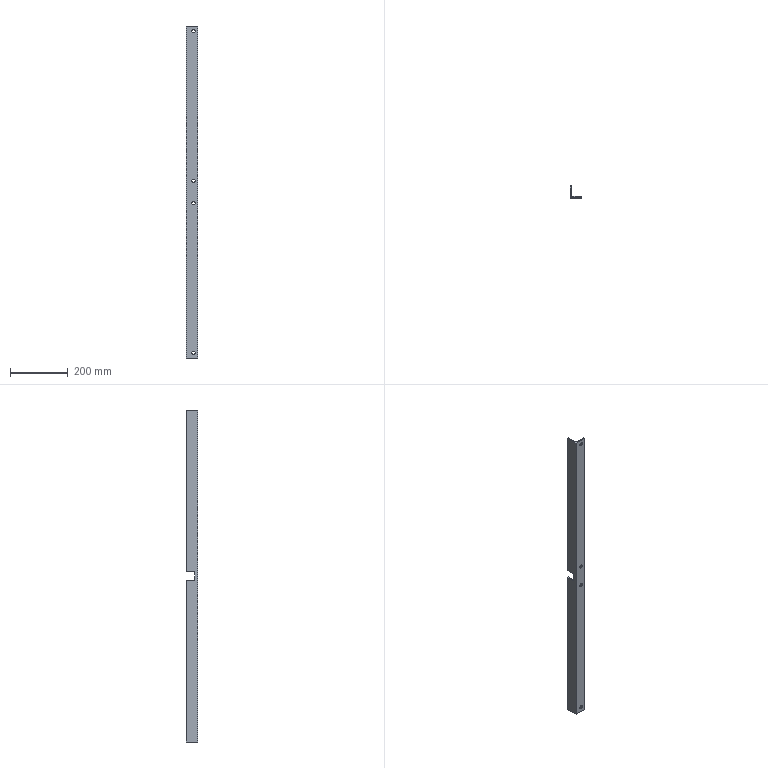Part | SolidWorks | features Extrusion 1, HoleWzd 1, ICE 1 | 1 solid | 24 faces | box 40 x 40 x 1150 mm | volume 350360 mm3 | cylinder 12 | plane 12 | commonest cylinder face diameters 12 x8 0.02 x3 10 x1
STEP:
#1=CARTESIAN_POINT('',(24.99,0.,1126.));
#2=VERTEX_POINT('',#1);
#3=CARTESIAN_POINT('',(24.99,0.,1138.));
#4=VERTEX_POINT('',#3);
#5=CARTESIAN_POINT('',(24.99,0.,1132.));
#6=DIRECTION('',(0.,1.,0.));
#7=DIRECTION('',(0.,0.,1.));
#8=AXIS2_PLACEMENT_3D('',#5,#6,#7);
#9=CIRCLE('',#8,6.);
#10=EDGE_CURVE('',#2,#4,#9,.T.);
#11=ORIENTED_EDGE('',*,*,#10,.F.);
#12=CARTESIAN_POINT('',(24.99,4.,1126.));
#13=VERTEX_POINT('',#12);
#14=CARTESIAN_POINT('',(24.99,4.,1126.));
#15=DIRECTION('',(0.,1.,0.));
#16=VECTOR('',#15,1000.);
#17=LINE('',#14,#16);
#18=EDGE_CURVE('',#2,#13,#17,.T.);
#19=ORIENTED_EDGE('',*,*,#18,.T.);
#20=CARTESIAN_POINT('',(24.99,4.,1138.));
#21=VERTEX_POINT('',#20);
#22=CARTESIAN_POINT('',(24.99,4.,1132.));
#23=DIRECTION('',(0.,1.,0.));
#24=DIRECTION('',(0.,0.,1.));
#25=AXIS2_PLACEMENT_3D('',#22,#23,#24);
#26=CIRCLE('',#25,6.);
#27=EDGE_CURVE('',#13,#21,#26,.T.);
#28=ORIENTED_EDGE('',*,*,#27,.T.);
#29=CARTESIAN_POINT('',(24.99,4.,1138.));
#30=DIRECTION('',(0.,1.,0.));
#31=VECTOR('',#30,1000.);
#32=LINE('',#29,#31);
#33=EDGE_CURVE('',#4,#21,#32,.T.);
#34=ORIENTED_EDGE('',*,*,#33,.F.);
#35=EDGE_LOOP('',(#11,#19,#28,#34));
#36=FACE_OUTER_BOUND('',#35,.T.);
#37=CARTESIAN_POINT('',(24.99,4.,1132.));
#38=DIRECTION('',(0.,1.,0.));
#39=DIRECTION('',(0.,0.,1.));
#40=AXIS2_PLACEMENT_3D('',#37,#38,#39);
#41=CYLINDRICAL_SURFACE('',#40,6.);
#42=ADVANCED_FACE('',(#36),#41,.F.);
#43=CARTESIAN_POINT('',(24.99,0.,608.));
#44=VERTEX_POINT('',#43);
#45=CARTESIAN_POINT('',(24.99,0.,620.));
#46=VERTEX_POINT('',#45);
#47=CARTESIAN_POINT('',(24.99,0.,614.));
#48=DIRECTION('',(0.,1.,0.));
#49=DIRECTION('',(0.,0.,1.));
#50=AXIS2_PLACEMENT_3D('',#47,#48,#49);
#51=CIRCLE('',#50,6.);
#52=EDGE_CURVE('',#44,#46,#51,.T.);
#53=ORIENTED_EDGE('',*,*,#52,.F.);
#54=CARTESIAN_POINT('',(24.99,4.,608.));
#55=VERTEX_POINT('',#54);
#56=CARTESIAN_POINT('',(24.99,4.,608.));
#57=DIRECTION('',(0.,1.,0.));
#58=VECTOR('',#57,1000.);
#59=LINE('',#56,#58);
#60=EDGE_CURVE('',#44,#55,#59,.T.);
#61=ORIENTED_EDGE('',*,*,#60,.T.);
#62=CARTESIAN_POINT('',(24.99,4.,620.));
#63=VERTEX_POINT('',#62);
#64=CARTESIAN_POINT('',(24.99,4.,614.));
#65=DIRECTION('',(0.,1.,0.));
#66=DIRECTION('',(0.,0.,1.));
#67=AXIS2_PLACEMENT_3D('',#64,#65,#66);
#68=CIRCLE('',#67,6.);
#69=EDGE_CURVE('',#55,#63,#68,.T.);
#70=ORIENTED_EDGE('',*,*,#69,.T.);
#71=CARTESIAN_POINT('',(24.99,4.,620.));
#72=DIRECTION('',(0.,1.,0.));
#73=VECTOR('',#72,1000.);
#74=LINE('',#71,#73);
#75=EDGE_CURVE('',#46,#63,#74,.T.);
#76=ORIENTED_EDGE('',*,*,#75,.F.);
#77=EDGE_LOOP('',(#53,#61,#70,#76));
#78=FACE_OUTER_BOUND('',#77,.T.);
#79=CARTESIAN_POINT('',(24.99,4.,614.));
#80=DIRECTION('',(0.,1.,0.));
#81=DIRECTION('',(0.,0.,1.));
#82=AXIS2_PLACEMENT_3D('',#79,#80,#81);
#83=CYLINDRICAL_SURFACE('',#82,6.);
#84=ADVANCED_FACE('',(#78),#83,.F.);
#85=CARTESIAN_POINT('',(24.99,0.,530.));
#86=VERTEX_POINT('',#85);
#87=CARTESIAN_POINT('',(24.99,0.,542.));
#88=VERTEX_POINT('',#87);
#89=CARTESIAN_POINT('',(24.99,0.,536.));
#90=DIRECTION('',(0.,1.,0.));
#91=DIRECTION('',(0.,0.,1.));
#92=AXIS2_PLACEMENT_3D('',#89,#90,#91);
#93=CIRCLE('',#92,6.);
#94=EDGE_CURVE('',#86,#88,#93,.T.);
#95=ORIENTED_EDGE('',*,*,#94,.F.);
#96=CARTESIAN_POINT('',(24.99,4.,530.));
#97=VERTEX_POINT('',#96);
#98=CARTESIAN_POINT('',(24.99,4.,530.));
#99=DIRECTION('',(0.,1.,0.));
#100=VECTOR('',#99,1000.);
#101=LINE('',#98,#100);
#102=EDGE_CURVE('',#86,#97,#101,.T.);
#103=ORIENTED_EDGE('',*,*,#102,.T.);
#104=CARTESIAN_POINT('',(24.99,4.,542.));
#105=VERTEX_POINT('',#104);
#106=CARTESIAN_POINT('',(24.99,4.,536.));
#107=DIRECTION('',(0.,1.,0.));
#108=DIRECTION('',(0.,0.,1.));
#109=AXIS2_PLACEMENT_3D('',#106,#107,#108);
#110=CIRCLE('',#109,6.);
#111=EDGE_CURVE('',#97,#105,#110,.T.);
#112=ORIENTED_EDGE('',*,*,#111,.T.);
#113=CARTESIAN_POINT('',(24.99,4.,542.));
#114=DIRECTION('',(0.,1.,0.));
#115=VECTOR('',#114,1000.);
#116=LINE('',#113,#115);
#117=EDGE_CURVE('',#88,#105,#116,.T.);
#118=ORIENTED_EDGE('',*,*,#117,.F.);
#119=EDGE_LOOP('',(#95,#103,#112,#118));
#120=FACE_OUTER_BOUND('',#119,.T.);
#121=CARTESIAN_POINT('',(24.99,4.,536.));
#122=DIRECTION('',(0.,1.,0.));
#123=DIRECTION('',(0.,0.,1.));
#124=AXIS2_PLACEMENT_3D('',#121,#122,#123);
#125=CYLINDRICAL_SURFACE('',#124,6.);
#126=ADVANCED_FACE('',(#120),#125,.F.);
#127=CARTESIAN_POINT('',(24.99,0.,12.));
#128=VERTEX_POINT('',#127);
#129=CARTESIAN_POINT('',(24.99,0.,24.));
#130=VERTEX_POINT('',#129);
#131=CARTESIAN_POINT('',(24.99,0.,18.));
#132=DIRECTION('',(0.,1.,0.));
#133=DIRECTION('',(0.,0.,1.));
#134=AXIS2_PLACEMENT_3D('',#131,#132,#133);
#135=CIRCLE('',#134,6.);
#136=EDGE_CURVE('',#128,#130,#135,.T.);
#137=ORIENTED_EDGE('',*,*,#136,.F.);
#138=CARTESIAN_POINT('',(24.99,4.,12.));
#139=VERTEX_POINT('',#138);
#140=CARTESIAN_POINT('',(24.99,4.,12.));
#141=DIRECTION('',(0.,1.,0.));
#142=VECTOR('',#141,1000.);
#143=LINE('',#140,#142);
#144=EDGE_CURVE('',#128,#139,#143,.T.);
#145=ORIENTED_EDGE('',*,*,#144,.T.);
#146=CARTESIAN_POINT('',(24.99,4.,24.));
#147=VERTEX_POINT('',#146);
#148=CARTESIAN_POINT('',(24.99,4.,18.));
#149=DIRECTION('',(0.,1.,0.));
#150=DIRECTION('',(0.,0.,1.));
#151=AXIS2_PLACEMENT_3D('',#148,#149,#150);
#152=CIRCLE('',#151,6.);
#153=EDGE_CURVE('',#139,#147,#152,.T.);
#154=ORIENTED_EDGE('',*,*,#153,.T.);
#155=CARTESIAN_POINT('',(24.99,4.,24.));
#156=DIRECTION('',(0.,1.,0.));
#157=VECTOR('',#156,1000.);
#158=LINE('',#155,#157);
#159=EDGE_CURVE('',#130,#147,#158,.T.);
#160=ORIENTED_EDGE('',*,*,#159,.F.);
#161=EDGE_LOOP('',(#137,#145,#154,#160));
#162=FACE_OUTER_BOUND('',#161,.T.);
#163=CARTESIAN_POINT('',(24.99,4.,18.));
#164=DIRECTION('',(0.,1.,0.));
#165=DIRECTION('',(0.,0.,1.));
#166=AXIS2_PLACEMENT_3D('',#163,#164,#165);
#167=CYLINDRICAL_SURFACE('',#166,6.);
#168=ADVANCED_FACE('',(#162),#167,.F.);
#169=CARTESIAN_POINT('',(4.,39.99,1150.));
#170=VERTEX_POINT('',#169);
#171=CARTESIAN_POINT('',(4.,39.99,590.));
#172=VERTEX_POINT('',#171);
#173=CARTESIAN_POINT('',(4.,39.99,1150.));
#174=DIRECTION('',(0.,0.,-1.));
#175=VECTOR('',#174,1000.);
#176=LINE('',#173,#175);
#177=EDGE_CURVE('',#170,#172,#176,.T.);
#178=ORIENTED_EDGE('',*,*,#177,.T.);
#179=CARTESIAN_POINT('',(3.99,40.,590.));
#180=VERTEX_POINT('',#179);
#181=CARTESIAN_POINT('',(3.99,39.99,590.));
#182=DIRECTION('',(0.,0.,1.));
#183=DIRECTION('',(1.,0.,0.));
#184=AXIS2_PLACEMENT_3D('',#181,#182,#183);
#185=CIRCLE('',#184,0.01);
#186=EDGE_CURVE('',#172,#180,#185,.T.);
#187=ORIENTED_EDGE('',*,*,#186,.T.);
#188=CARTESIAN_POINT('',(3.99,40.,1150.));
#189=VERTEX_POINT('',#188);
#190=CARTESIAN_POINT('',(3.99,40.,1150.));
#191=DIRECTION('',(0.,0.,-1.));
#192=VECTOR('',#191,1000.);
#193=LINE('',#190,#192);
#194=EDGE_CURVE('',#189,#180,#193,.T.);
#195=ORIENTED_EDGE('',*,*,#194,.F.);
#196=CARTESIAN_POINT('',(3.99,39.99,1150.));
#197=DIRECTION('',(0.,0.,1.));
#198=DIRECTION('',(1.,0.,0.));
#199=AXIS2_PLACEMENT_3D('',#196,#197,#198);
#200=CIRCLE('',#199,0.01);
#201=EDGE_CURVE('',#170,#189,#200,.T.);
#202=ORIENTED_EDGE('',*,*,#201,.F.);
#203=EDGE_LOOP('',(#178,#187,#195,#202));
#204=FACE_OUTER_BOUND('',#203,.T.);
#205=CARTESIAN_POINT('',(3.99,39.99,1150.));
#206=DIRECTION('',(0.,0.,-1.));
#207=DIRECTION('',(-1.,0.,0.));
#208=AXIS2_PLACEMENT_3D('',#205,#206,#207);
#209=CYLINDRICAL_SURFACE('',#208,0.01);
#210=ADVANCED_FACE('',(#204),#209,.T.);
#211=ORIENTED_EDGE('',*,*,#194,.T.);
#212=CARTESIAN_POINT('',(0.,40.,590.));
#213=VERTEX_POINT('',#212);
#214=CARTESIAN_POINT('',(0.,40.,590.));
#215=DIRECTION('',(-1.,0.,0.));
#216=VECTOR('',#215,1000.);
#217=LINE('',#214,#216);
#218=EDGE_CURVE('',#180,#213,#217,.T.);
#219=ORIENTED_EDGE('',*,*,#218,.T.);
#220=CARTESIAN_POINT('',(0.,40.,1150.));
#221=VERTEX_POINT('',#220);
#222=CARTESIAN_POINT('',(0.,40.,1150.));
#223=DIRECTION('',(0.,0.,-1.));
#224=VECTOR('',#223,1000.);
#225=LINE('',#222,#224);
#226=EDGE_CURVE('',#221,#213,#225,.T.);
#227=ORIENTED_EDGE('',*,*,#226,.F.);
#228=CARTESIAN_POINT('',(0.,40.,1150.));
#229=DIRECTION('',(-1.,0.,0.));
#230=VECTOR('',#229,1000.);
#231=LINE('',#228,#230);
#232=EDGE_CURVE('',#189,#221,#231,.T.);
#233=ORIENTED_EDGE('',*,*,#232,.F.);
#234=EDGE_LOOP('',(#211,#219,#227,#233));
#235=FACE_OUTER_BOUND('',#234,.T.);
#236=CARTESIAN_POINT('',(0.,40.,1150.));
#237=DIRECTION('',(0.,-1.,0.));
#238=DIRECTION('',(0.,0.,-1.));
#239=AXIS2_PLACEMENT_3D('',#236,#237,#238);
#240=PLANE('',#239);
#241=ADVANCED_FACE('',(#235),#240,.F.);
#242=CARTESIAN_POINT('',(24.99,0.,1132.));
#243=DIRECTION('',(0.,1.,0.));
#244=DIRECTION('',(0.,0.,1.));
#245=AXIS2_PLACEMENT_3D('',#242,#243,#244);
#246=CIRCLE('',#245,6.);
#247=EDGE_CURVE('',#4,#2,#246,.T.);
#248=ORIENTED_EDGE('',*,*,#247,.T.);
#249=ORIENTED_EDGE('',*,*,#10,.T.);
#250=EDGE_LOOP('',(#248,#249));
#251=FACE_BOUND('',#250,.T.);
#252=CARTESIAN_POINT('',(24.99,0.,614.));
#253=DIRECTION('',(0.,1.,0.));
#254=DIRECTION('',(0.,0.,1.));
#255=AXIS2_PLACEMENT_3D('',#252,#253,#254);
#256=CIRCLE('',#255,6.);
#257=EDGE_CURVE('',#46,#44,#256,.T.);
#258=ORIENTED_EDGE('',*,*,#257,.T.);
#259=ORIENTED_EDGE('',*,*,#52,.T.);
#260=EDGE_LOOP('',(#258,#259));
#261=FACE_BOUND('',#260,.T.);
#262=CARTESIAN_POINT('',(24.99,0.,536.));
#263=DIRECTION('',(0.,1.,0.));
#264=DIRECTION('',(0.,0.,1.));
#265=AXIS2_PLACEMENT_3D('',#262,#263,#264);
#266=CIRCLE('',#265,6.);
#267=EDGE_CURVE('',#88,#86,#266,.T.);
#268=ORIENTED_EDGE('',*,*,#267,.T.);
#269=ORIENTED_EDGE('',*,*,#94,.T.);
#270=EDGE_LOOP('',(#268,#269));
#271=FACE_BOUND('',#270,.T.);
#272=CARTESIAN_POINT('',(24.99,0.,18.));
#273=DIRECTION('',(0.,1.,0.));
#274=DIRECTION('',(0.,0.,1.));
#275=AXIS2_PLACEMENT_3D('',#272,#273,#274);
#276=CIRCLE('',#275,6.);
#277=EDGE_CURVE('',#130,#128,#276,.T.);
#278=ORIENTED_EDGE('',*,*,#277,.T.);
#279=ORIENTED_EDGE('',*,*,#136,.T.);
#280=EDGE_LOOP('',(#278,#279));
#281=FACE_BOUND('',#280,.T.);
#282=CARTESIAN_POINT('',(0.,0.,0.));
#283=VERTEX_POINT('',#282);
#284=CARTESIAN_POINT('',(40.,0.,0.));
#285=VERTEX_POINT('',#284);
#286=CARTESIAN_POINT('',(40.,0.,0.));
#287=DIRECTION('',(1.,0.,0.));
#288=VECTOR('',#287,1000.);
#289=LINE('',#286,#288);
#290=EDGE_CURVE('',#283,#285,#289,.T.);
#291=ORIENTED_EDGE('',*,*,#290,.T.);
#292=CARTESIAN_POINT('',(40.,0.,1150.));
#293=VERTEX_POINT('',#292);
#294=CARTESIAN_POINT('',(40.,0.,1150.));
#295=DIRECTION('',(0.,0.,-1.));
#296=VECTOR('',#295,1000.);
#297=LINE('',#294,#296);
#298=EDGE_CURVE('',#293,#285,#297,.T.);
#299=ORIENTED_EDGE('',*,*,#298,.F.);
#300=CARTESIAN_POINT('',(0.,0.,1150.));
#301=VERTEX_POINT('',#300);
#302=CARTESIAN_POINT('',(40.,0.,1150.));
#303=DIRECTION('',(1.,0.,0.));
#304=VECTOR('',#303,1000.);
#305=LINE('',#302,#304);
#306=EDGE_CURVE('',#301,#293,#305,.T.);
#307=ORIENTED_EDGE('',*,*,#306,.F.);
#308=CARTESIAN_POINT('',(0.,0.,1150.));
#309=DIRECTION('',(0.,0.,-1.));
#310=VECTOR('',#309,1000.);
#311=LINE('',#308,#310);
#312=EDGE_CURVE('',#301,#283,#311,.T.);
#313=ORIENTED_EDGE('',*,*,#312,.T.);
#314=EDGE_LOOP('',(#291,#299,#307,#313));
#315=FACE_OUTER_BOUND('',#314,.T.);
#316=CARTESIAN_POINT('',(40.,0.,1150.));
#317=DIRECTION('',(0.,1.,0.));
#318=DIRECTION('',(-1.,0.,0.));
#319=AXIS2_PLACEMENT_3D('',#316,#317,#318);
#320=PLANE('',#319);
#321=ADVANCED_FACE('',(#251,#261,#271,#281,#315),#320,.F.);
#322=CARTESIAN_POINT('',(40.,3.99,0.));
#323=VERTEX_POINT('',#322);
#324=CARTESIAN_POINT('',(40.,3.99,0.));
#325=DIRECTION('',(0.,1.,0.));
#326=VECTOR('',#325,1000.);
#327=LINE('',#324,#326);
#328=EDGE_CURVE('',#285,#323,#327,.T.);
#329=ORIENTED_EDGE('',*,*,#328,.T.);
#330=CARTESIAN_POINT('',(40.,3.99,1150.));
#331=VERTEX_POINT('',#330);
#332=CARTESIAN_POINT('',(40.,3.99,1150.));
#333=DIRECTION('',(0.,0.,-1.));
#334=VECTOR('',#333,1000.);
#335=LINE('',#332,#334);
#336=EDGE_CURVE('',#331,#323,#335,.T.);
#337=ORIENTED_EDGE('',*,*,#336,.F.);
#338=CARTESIAN_POINT('',(40.,3.99,1150.));
#339=DIRECTION('',(0.,1.,0.));
#340=VECTOR('',#339,1000.);
#341=LINE('',#338,#340);
#342=EDGE_CURVE('',#293,#331,#341,.T.);
#343=ORIENTED_EDGE('',*,*,#342,.F.);
#344=ORIENTED_EDGE('',*,*,#298,.T.);
#345=EDGE_LOOP('',(#329,#337,#343,#344));
#346=FACE_OUTER_BOUND('',#345,.T.);
#347=CARTESIAN_POINT('',(40.,3.99,1150.));
#348=DIRECTION('',(-1.,0.,0.));
#349=DIRECTION('',(0.,-1.,0.));
#350=AXIS2_PLACEMENT_3D('',#347,#348,#349);
#351=PLANE('',#350);
#352=ADVANCED_FACE('',(#346),#351,.F.);
#353=CARTESIAN_POINT('',(39.99,4.,0.));
#354=VERTEX_POINT('',#353);
#355=CARTESIAN_POINT('',(39.99,3.99,0.));
#356=DIRECTION('',(0.,0.,1.));
#357=DIRECTION('',(1.,0.,0.));
#358=AXIS2_PLACEMENT_3D('',#355,#356,#357);
#359=CIRCLE('',#358,0.01);
#360=EDGE_CURVE('',#323,#354,#359,.T.);
#361=ORIENTED_EDGE('',*,*,#360,.T.);
#362=CARTESIAN_POINT('',(39.99,4.,1150.));
#363=VERTEX_POINT('',#362);
#364=CARTESIAN_POINT('',(39.99,4.,1150.));
#365=DIRECTION('',(0.,0.,-1.));
#366=VECTOR('',#365,1000.);
#367=LINE('',#364,#366);
#368=EDGE_CURVE('',#363,#354,#367,.T.);
#369=ORIENTED_EDGE('',*,*,#368,.F.);
#370=CARTESIAN_POINT('',(39.99,3.99,1150.));
#371=DIRECTION('',(0.,0.,1.));
#372=DIRECTION('',(1.,0.,0.));
#373=AXIS2_PLACEMENT_3D('',#370,#371,#372);
#374=CIRCLE('',#373,0.01);
#375=EDGE_CURVE('',#331,#363,#374,.T.);
#376=ORIENTED_EDGE('',*,*,#375,.F.);
#377=ORIENTED_EDGE('',*,*,#336,.T.);
#378=EDGE_LOOP('',(#361,#369,#376,#377));
#379=FACE_OUTER_BOUND('',#378,.T.);
#380=CARTESIAN_POINT('',(39.99,3.99,1150.));
#381=DIRECTION('',(0.,0.,-1.));
#382=DIRECTION('',(-1.,0.,0.));
#383=AXIS2_PLACEMENT_3D('',#380,#381,#382);
#384=CYLINDRICAL_SURFACE('',#383,0.01);
#385=ADVANCED_FACE('',(#379),#384,.T.);
#386=CARTESIAN_POINT('',(24.99,4.,1132.));
#387=DIRECTION('',(0.,1.,0.));
#388=DIRECTION('',(0.,0.,1.));
#389=AXIS2_PLACEMENT_3D('',#386,#387,#388);
#390=CIRCLE('',#389,6.);
#391=EDGE_CURVE('',#21,#13,#390,.T.);
#392=ORIENTED_EDGE('',*,*,#391,.F.);
#393=ORIENTED_EDGE('',*,*,#27,.F.);
#394=EDGE_LOOP('',(#392,#393));
#395=FACE_BOUND('',#394,.T.);
#396=CARTESIAN_POINT('',(24.99,4.,614.));
#397=DIRECTION('',(0.,1.,0.));
#398=DIRECTION('',(0.,0.,1.));
#399=AXIS2_PLACEMENT_3D('',#396,#397,#398);
#400=CIRCLE('',#399,6.);
#401=EDGE_CURVE('',#63,#55,#400,.T.);
#402=ORIENTED_EDGE('',*,*,#401,.F.);
#403=ORIENTED_EDGE('',*,*,#69,.F.);
#404=EDGE_LOOP('',(#402,#403));
#405=FACE_BOUND('',#404,.T.);
#406=CARTESIAN_POINT('',(24.99,4.,536.));
#407=DIRECTION('',(0.,1.,0.));
#408=DIRECTION('',(0.,0.,1.));
#409=AXIS2_PLACEMENT_3D('',#406,#407,#408);
#410=CIRCLE('',#409,6.);
#411=EDGE_CURVE('',#105,#97,#410,.T.);
#412=ORIENTED_EDGE('',*,*,#411,.F.);
#413=ORIENTED_EDGE('',*,*,#111,.F.);
#414=EDGE_LOOP('',(#412,#413));
#415=FACE_BOUND('',#414,.T.);
#416=CARTESIAN_POINT('',(24.99,4.,18.));
#417=DIRECTION('',(0.,1.,0.));
#418=DIRECTION('',(0.,0.,1.));
#419=AXIS2_PLACEMENT_3D('',#416,#417,#418);
#420=CIRCLE('',#419,6.);
#421=EDGE_CURVE('',#147,#139,#420,.T.);
#422=ORIENTED_EDGE('',*,*,#421,.F.);
#423=ORIENTED_EDGE('',*,*,#153,.F.);
#424=EDGE_LOOP('',(#422,#423));
#425=FACE_BOUND('',#424,.T.);
#426=CARTESIAN_POINT('',(9.,4.,0.));
#427=VERTEX_POINT('',#426);
#428=CARTESIAN_POINT('',(9.,4.,0.));
#429=DIRECTION('',(-1.,0.,0.));
#430=VECTOR('',#429,1000.);
#431=LINE('',#428,#430);
#432=EDGE_CURVE('',#354,#427,#431,.T.);
#433=ORIENTED_EDGE('',*,*,#432,.T.);
#434=CARTESIAN_POINT('',(9.,4.,1150.));
#435=VERTEX_POINT('',#434);
#436=CARTESIAN_POINT('',(9.,4.,1150.));
#437=DIRECTION('',(0.,0.,-1.));
#438=VECTOR('',#437,1000.);
#439=LINE('',#436,#438);
#440=EDGE_CURVE('',#435,#427,#439,.T.);
#441=ORIENTED_EDGE('',*,*,#440,.F.);
#442=CARTESIAN_POINT('',(9.,4.,1150.));
#443=DIRECTION('',(-1.,0.,0.));
#444=VECTOR('',#443,1000.);
#445=LINE('',#442,#444);
#446=EDGE_CURVE('',#363,#435,#445,.T.);
#447=ORIENTED_EDGE('',*,*,#446,.F.);
#448=ORIENTED_EDGE('',*,*,#368,.T.);
#449=EDGE_LOOP('',(#433,#441,#447,#448));
#450=FACE_OUTER_BOUND('',#449,.T.);
#451=CARTESIAN_POINT('',(9.,4.,1150.));
#452=DIRECTION('',(0.,-1.,0.));
#453=DIRECTION('',(1.,0.,0.));
#454=AXIS2_PLACEMENT_3D('',#451,#452,#453);
#455=PLANE('',#454);
#456=ADVANCED_FACE('',(#395,#405,#415,#425,#450),#455,.F.);
#457=CARTESIAN_POINT('',(4.,9.,0.));
#458=VERTEX_POINT('',#457);
#459=CARTESIAN_POINT('',(9.,9.,0.));
#460=DIRECTION('',(0.,0.,-1.));
#461=DIRECTION('',(-1.,0.,0.));
#462=AXIS2_PLACEMENT_3D('',#459,#460,#461);
#463=CIRCLE('',#462,5.);
#464=EDGE_CURVE('',#427,#458,#463,.T.);
#465=ORIENTED_EDGE('',*,*,#464,.T.);
#466=CARTESIAN_POINT('',(4.,9.,1150.));
#467=VERTEX_POINT('',#466);
#468=CARTESIAN_POINT('',(4.,9.,1150.));
#469=DIRECTION('',(0.,0.,-1.));
#470=VECTOR('',#469,1000.);
#471=LINE('',#468,#470);
#472=EDGE_CURVE('',#467,#458,#471,.T.);
#473=ORIENTED_EDGE('',*,*,#472,.F.);
#474=CARTESIAN_POINT('',(9.,9.,1150.));
#475=DIRECTION('',(0.,0.,-1.));
#476=DIRECTION('',(-1.,0.,0.));
#477=AXIS2_PLACEMENT_3D('',#474,#475,#476);
#478=CIRCLE('',#477,5.);
#479=EDGE_CURVE('',#435,#467,#478,.T.);
#480=ORIENTED_EDGE('',*,*,#479,.F.);
#481=ORIENTED_EDGE('',*,*,#440,.T.);
#482=EDGE_LOOP('',(#465,#473,#480,#481));
#483=FACE_OUTER_BOUND('',#482,.T.);
#484=CARTESIAN_POINT('',(9.,9.,1150.));
#485=DIRECTION('',(0.,0.,-1.));
#486=DIRECTION('',(-1.,0.,0.));
#487=AXIS2_PLACEMENT_3D('',#484,#485,#486);
#488=CYLINDRICAL_SURFACE('',#487,5.);
#489=ADVANCED_FACE('',(#483),#488,.F.);
#490=CARTESIAN_POINT('',(4.,10.,590.));
#491=VERTEX_POINT('',#490);
#492=CARTESIAN_POINT('',(4.,10.,560.));
#493=VERTEX_POINT('',#492);
#494=CARTESIAN_POINT('',(4.,10.,590.));
#495=DIRECTION('',(0.,0.,-1.));
#496=VECTOR('',#495,1000.);
#497=LINE('',#494,#496);
#498=EDGE_CURVE('',#491,#493,#497,.T.);
#499=ORIENTED_EDGE('',*,*,#498,.F.);
#500=CARTESIAN_POINT('',(4.,60.481,590.));
#501=DIRECTION('',(0.,-1.,0.));
#502=VECTOR('',#501,1000.);
#503=LINE('',#500,#502);
#504=EDGE_CURVE('',#172,#491,#503,.T.);
#505=ORIENTED_EDGE('',*,*,#504,.F.);
#506=ORIENTED_EDGE('',*,*,#177,.F.);
#507=CARTESIAN_POINT('',(4.,39.99,1150.));
#508=DIRECTION('',(0.,1.,0.));
#509=VECTOR('',#508,1000.);
#510=LINE('',#507,#509);
#511=EDGE_CURVE('',#467,#170,#510,.T.);
#512=ORIENTED_EDGE('',*,*,#511,.F.);
#513=ORIENTED_EDGE('',*,*,#472,.T.);
#514=CARTESIAN_POINT('',(4.,39.99,0.));
#515=VERTEX_POINT('',#514);
#516=CARTESIAN_POINT('',(4.,39.99,0.));
#517=DIRECTION('',(0.,1.,0.));
#518=VECTOR('',#517,1000.);
#519=LINE('',#516,#518);
#520=EDGE_CURVE('',#458,#515,#519,.T.);
#521=ORIENTED_EDGE('',*,*,#520,.T.);
#522=CARTESIAN_POINT('',(4.,39.99,560.));
#523=VERTEX_POINT('',#522);
#524=CARTESIAN_POINT('',(4.,39.99,1150.));
#525=DIRECTION('',(0.,0.,-1.));
#526=VECTOR('',#525,1000.);
#527=LINE('',#524,#526);
#528=EDGE_CURVE('',#523,#515,#527,.T.);
#529=ORIENTED_EDGE('',*,*,#528,.F.);
#530=CARTESIAN_POINT('',(4.,60.481,560.));
#531=DIRECTION('',(0.,1.,0.));
#532=VECTOR('',#531,1000.);
#533=LINE('',#530,#532);
#534=EDGE_CURVE('',#493,#523,#533,.T.);
#535=ORIENTED_EDGE('',*,*,#534,.F.);
#536=EDGE_LOOP('',(#499,#505,#506,#512,#513,#521,#529,#535));
#537=FACE_OUTER_BOUND('',#536,.T.);
#538=CARTESIAN_POINT('',(4.,39.99,1150.));
#539=DIRECTION('',(-1.,0.,0.));
#540=DIRECTION('',(0.,-1.,0.));
#541=AXIS2_PLACEMENT_3D('',#538,#539,#540);
#542=PLANE('',#541);
#543=ADVANCED_FACE('',(#537),#542,.F.);
#544=CARTESIAN_POINT('',(3.99,40.,560.));
#545=VERTEX_POINT('',#544);
#546=CARTESIAN_POINT('',(3.99,40.,0.));
#547=VERTEX_POINT('',#546);
#548=CARTESIAN_POINT('',(3.99,40.,1150.));
#549=DIRECTION('',(0.,0.,-1.));
#550=VECTOR('',#549,1000.);
#551=LINE('',#548,#550);
#552=EDGE_CURVE('',#545,#547,#551,.T.);
#553=ORIENTED_EDGE('',*,*,#552,.F.);
#554=CARTESIAN_POINT('',(3.99,39.99,560.));
#555=DIRECTION('',(0.,0.,-1.));
#556=DIRECTION('',(-1.,0.,0.));
#557=AXIS2_PLACEMENT_3D('',#554,#555,#556);
#558=CIRCLE('',#557,0.01);
#559=EDGE_CURVE('',#545,#523,#558,.T.);
#560=ORIENTED_EDGE('',*,*,#559,.T.);
#561=ORIENTED_EDGE('',*,*,#528,.T.);
#562=CARTESIAN_POINT('',(3.99,39.99,0.));
#563=DIRECTION('',(0.,0.,1.));
#564=DIRECTION('',(1.,0.,0.));
#565=AXIS2_PLACEMENT_3D('',#562,#563,#564);
#566=CIRCLE('',#565,0.01);
#567=EDGE_CURVE('',#515,#547,#566,.T.);
#568=ORIENTED_EDGE('',*,*,#567,.T.);
#569=EDGE_LOOP('',(#553,#560,#561,#568));
#570=FACE_OUTER_BOUND('',#569,.T.);
#571=CARTESIAN_POINT('',(3.99,39.99,1150.));
#572=DIRECTION('',(0.,0.,-1.));
#573=DIRECTION('',(-1.,0.,0.));
#574=AXIS2_PLACEMENT_3D('',#571,#572,#573);
#575=CYLINDRICAL_SURFACE('',#574,0.01);
#576=ADVANCED_FACE('',(#570),#575,.T.);
#577=CARTESIAN_POINT('',(0.,40.,560.));
#578=VERTEX_POINT('',#577);
#579=CARTESIAN_POINT('',(0.,40.,0.));
#580=VERTEX_POINT('',#579);
#581=CARTESIAN_POINT('',(0.,40.,1150.));
#582=DIRECTION('',(0.,0.,-1.));
#583=VECTOR('',#582,1000.);
#584=LINE('',#581,#583);
#585=EDGE_CURVE('',#578,#580,#584,.T.);
#586=ORIENTED_EDGE('',*,*,#585,.F.);
#587=CARTESIAN_POINT('',(0.,40.,560.));
#588=DIRECTION('',(1.,0.,0.));
#589=VECTOR('',#588,1000.);
#590=LINE('',#587,#589);
#591=EDGE_CURVE('',#578,#545,#590,.T.);
#592=ORIENTED_EDGE('',*,*,#591,.T.);
#593=ORIENTED_EDGE('',*,*,#552,.T.);
#594=CARTESIAN_POINT('',(0.,40.,0.));
#595=DIRECTION('',(-1.,0.,0.));
#596=VECTOR('',#595,1000.);
#597=LINE('',#594,#596);
#598=EDGE_CURVE('',#547,#580,#597,.T.);
#599=ORIENTED_EDGE('',*,*,#598,.T.);
#600=EDGE_LOOP('',(#586,#592,#593,#599));
#601=FACE_OUTER_BOUND('',#600,.T.);
#602=CARTESIAN_POINT('',(0.,40.,1150.));
#603=DIRECTION('',(0.,-1.,0.));
#604=DIRECTION('',(0.,0.,-1.));
#605=AXIS2_PLACEMENT_3D('',#602,#603,#604);
#606=PLANE('',#605);
#607=ADVANCED_FACE('',(#601),#606,.F.);
#608=ORIENTED_EDGE('',*,*,#226,.T.);
#609=CARTESIAN_POINT('',(0.,10.,590.));
#610=VERTEX_POINT('',#609);
#611=CARTESIAN_POINT('',(0.,0.,590.));
#612=DIRECTION('',(0.,-1.,0.));
#613=VECTOR('',#612,1000.);
#614=LINE('',#611,#613);
#615=EDGE_CURVE('',#213,#610,#614,.T.);
#616=ORIENTED_EDGE('',*,*,#615,.T.);
#617=CARTESIAN_POINT('',(0.,10.,560.));
#618=VERTEX_POINT('',#617);
#619=CARTESIAN_POINT('',(0.,10.,1150.));
#620=DIRECTION('',(0.,0.,-1.));
#621=VECTOR('',#620,1000.);
#622=LINE('',#619,#621);
#623=EDGE_CURVE('',#610,#618,#622,.T.);
#624=ORIENTED_EDGE('',*,*,#623,.T.);
#625=CARTESIAN_POINT('',(0.,0.,560.));
#626=DIRECTION('',(0.,1.,0.));
#627=VECTOR('',#626,1000.);
#628=LINE('',#625,#627);
#629=EDGE_CURVE('',#618,#578,#628,.T.);
#630=ORIENTED_EDGE('',*,*,#629,.T.);
#631=ORIENTED_EDGE('',*,*,#585,.T.);
#632=CARTESIAN_POINT('',(0.,0.,0.));
#633=DIRECTION('',(0.,-1.,0.));
#634=VECTOR('',#633,1000.);
#635=LINE('',#632,#634);
#636=EDGE_CURVE('',#580,#283,#635,.T.);
#637=ORIENTED_EDGE('',*,*,#636,.T.);
#638=ORIENTED_EDGE('',*,*,#312,.F.);
#639=CARTESIAN_POINT('',(0.,0.,1150.));
#640=DIRECTION('',(0.,-1.,0.));
#641=VECTOR('',#640,1000.);
#642=LINE('',#639,#641);
#643=EDGE_CURVE('',#221,#301,#642,.T.);
#644=ORIENTED_EDGE('',*,*,#643,.F.);
#645=EDGE_LOOP('',(#608,#616,#624,#630,#631,#637,#638,#644));
#646=FACE_OUTER_BOUND('',#645,.T.);
#647=CARTESIAN_POINT('',(0.,0.,1150.));
#648=DIRECTION('',(1.,0.,0.));
#649=DIRECTION('',(0.,0.,-1.));
#650=AXIS2_PLACEMENT_3D('',#647,#648,#649);
#651=PLANE('',#650);
#652=ADVANCED_FACE('',(#646),#651,.F.);
#653=ORIENTED_EDGE('',*,*,#306,.T.);
#654=ORIENTED_EDGE('',*,*,#342,.T.);
#655=ORIENTED_EDGE('',*,*,#375,.T.);
#656=ORIENTED_EDGE('',*,*,#446,.T.);
#657=ORIENTED_EDGE('',*,*,#479,.T.);
#658=ORIENTED_EDGE('',*,*,#511,.T.);
#659=ORIENTED_EDGE('',*,*,#201,.T.);
#660=ORIENTED_EDGE('',*,*,#232,.T.);
#661=ORIENTED_EDGE('',*,*,#643,.T.);
#662=EDGE_LOOP('',(#653,#654,#655,#656,#657,#658,#659,#660,#661));
#663=FACE_OUTER_BOUND('',#662,.T.);
#664=CARTESIAN_POINT('',(3.99,39.99,1150.));
#665=DIRECTION('',(0.,0.,1.));
#666=DIRECTION('',(1.,0.,0.));
#667=AXIS2_PLACEMENT_3D('',#664,#665,#666);
#668=PLANE('',#667);
#669=ADVANCED_FACE('',(#663),#668,.T.);
#670=ORIENTED_EDGE('',*,*,#290,.F.);
#671=ORIENTED_EDGE('',*,*,#636,.F.);
#672=ORIENTED_EDGE('',*,*,#598,.F.);
#673=ORIENTED_EDGE('',*,*,#567,.F.);
#674=ORIENTED_EDGE('',*,*,#520,.F.);
#675=ORIENTED_EDGE('',*,*,#464,.F.);
#676=ORIENTED_EDGE('',*,*,#432,.F.);
#677=ORIENTED_EDGE('',*,*,#360,.F.);
#678=ORIENTED_EDGE('',*,*,#328,.F.);
#679=EDGE_LOOP('',(#670,#671,#672,#673,#674,#675,#676,#677,#678));
#680=FACE_OUTER_BOUND('',#679,.T.);
#681=CARTESIAN_POINT('',(3.99,39.99,0.));
#682=DIRECTION('',(0.,0.,1.));
#683=DIRECTION('',(1.,0.,0.));
#684=AXIS2_PLACEMENT_3D('',#681,#682,#683);
#685=PLANE('',#684);
#686=ADVANCED_FACE('',(#680),#685,.F.);
#687=ORIENTED_EDGE('',*,*,#144,.F.);
#688=ORIENTED_EDGE('',*,*,#277,.F.);
#689=ORIENTED_EDGE('',*,*,#159,.T.);
#690=ORIENTED_EDGE('',*,*,#421,.T.);
#691=EDGE_LOOP('',(#687,#688,#689,#690));
#692=FACE_OUTER_BOUND('',#691,.T.);
#693=CARTESIAN_POINT('',(24.99,4.,18.));
#694=DIRECTION('',(0.,1.,0.));
#695=DIRECTION('',(0.,0.,1.));
#696=AXIS2_PLACEMENT_3D('',#693,#694,#695);
#697=CYLINDRICAL_SURFACE('',#696,6.);
#698=ADVANCED_FACE('',(#692),#697,.F.);
#699=ORIENTED_EDGE('',*,*,#102,.F.);
#700=ORIENTED_EDGE('',*,*,#267,.F.);
#701=ORIENTED_EDGE('',*,*,#117,.T.);
#702=ORIENTED_EDGE('',*,*,#411,.T.);
#703=EDGE_LOOP('',(#699,#700,#701,#702));
#704=FACE_OUTER_BOUND('',#703,.T.);
#705=CARTESIAN_POINT('',(24.99,4.,536.));
#706=DIRECTION('',(0.,1.,0.));
#707=DIRECTION('',(0.,0.,1.));
#708=AXIS2_PLACEMENT_3D('',#705,#706,#707);
#709=CYLINDRICAL_SURFACE('',#708,6.);
#710=ADVANCED_FACE('',(#704),#709,.F.);
#711=ORIENTED_EDGE('',*,*,#60,.F.);
#712=ORIENTED_EDGE('',*,*,#257,.F.);
#713=ORIENTED_EDGE('',*,*,#75,.T.);
#714=ORIENTED_EDGE('',*,*,#401,.T.);
#715=EDGE_LOOP('',(#711,#712,#713,#714));
#716=FACE_OUTER_BOUND('',#715,.T.);
#717=CARTESIAN_POINT('',(24.99,4.,614.));
#718=DIRECTION('',(0.,1.,0.));
#719=DIRECTION('',(0.,0.,1.));
#720=AXIS2_PLACEMENT_3D('',#717,#718,#719);
#721=CYLINDRICAL_SURFACE('',#720,6.);
#722=ADVANCED_FACE('',(#716),#721,.F.);
#723=ORIENTED_EDGE('',*,*,#18,.F.);
#724=ORIENTED_EDGE('',*,*,#247,.F.);
#725=ORIENTED_EDGE('',*,*,#33,.T.);
#726=ORIENTED_EDGE('',*,*,#391,.T.);
#727=EDGE_LOOP('',(#723,#724,#725,#726));
#728=FACE_OUTER_BOUND('',#727,.T.);
#729=CARTESIAN_POINT('',(24.99,4.,1132.));
#730=DIRECTION('',(0.,1.,0.));
#731=DIRECTION('',(0.,0.,1.));
#732=AXIS2_PLACEMENT_3D('',#729,#730,#731);
#733=CYLINDRICAL_SURFACE('',#732,6.);
#734=ADVANCED_FACE('',(#728),#733,.F.);
#735=ORIENTED_EDGE('',*,*,#504,.T.);
#736=CARTESIAN_POINT('',(-6.,10.,590.));
#737=DIRECTION('',(1.,0.,0.));
#738=VECTOR('',#737,1000.);
#739=LINE('',#736,#738);
#740=EDGE_CURVE('',#610,#491,#739,.T.);
#741=ORIENTED_EDGE('',*,*,#740,.F.);
#742=ORIENTED_EDGE('',*,*,#615,.F.);
#743=ORIENTED_EDGE('',*,*,#218,.F.);
#744=ORIENTED_EDGE('',*,*,#186,.F.);
#745=EDGE_LOOP('',(#735,#741,#742,#743,#744));
#746=FACE_OUTER_BOUND('',#745,.T.);
#747=CARTESIAN_POINT('',(-6.,60.481,590.));
#748=DIRECTION('',(0.,0.,1.));
#749=DIRECTION('',(1.,0.,0.));
#750=AXIS2_PLACEMENT_3D('',#747,#748,#749);
#751=PLANE('',#750);
#752=ADVANCED_FACE('',(#746),#751,.F.);
#753=ORIENTED_EDGE('',*,*,#591,.F.);
#754=ORIENTED_EDGE('',*,*,#629,.F.);
#755=CARTESIAN_POINT('',(-6.,10.,560.));
#756=DIRECTION('',(1.,0.,0.));
#757=VECTOR('',#756,1000.);
#758=LINE('',#755,#757);
#759=EDGE_CURVE('',#618,#493,#758,.T.);
#760=ORIENTED_EDGE('',*,*,#759,.T.);
#761=ORIENTED_EDGE('',*,*,#534,.T.);
#762=ORIENTED_EDGE('',*,*,#559,.F.);
#763=EDGE_LOOP('',(#753,#754,#760,#761,#762));
#764=FACE_OUTER_BOUND('',#763,.T.);
#765=CARTESIAN_POINT('',(-6.,60.481,560.));
#766=DIRECTION('',(0.,0.,-1.));
#767=DIRECTION('',(-1.,0.,0.));
#768=AXIS2_PLACEMENT_3D('',#765,#766,#767);
#769=PLANE('',#768);
#770=ADVANCED_FACE('',(#764),#769,.F.);
#771=ORIENTED_EDGE('',*,*,#740,.T.);
#772=ORIENTED_EDGE('',*,*,#498,.T.);
#773=ORIENTED_EDGE('',*,*,#759,.F.);
#774=ORIENTED_EDGE('',*,*,#623,.F.);
#775=EDGE_LOOP('',(#771,#772,#773,#774));
#776=FACE_OUTER_BOUND('',#775,.T.);
#777=CARTESIAN_POINT('',(-6.,10.,590.));
#778=DIRECTION('',(0.,-1.,0.));
#779=DIRECTION('',(1.,0.,0.));
#780=AXIS2_PLACEMENT_3D('',#777,#778,#779);
#781=PLANE('',#780);
#782=ADVANCED_FACE('',(#776),#781,.F.);
#783=CLOSED_SHELL('',(#42,#84,#126,#168,#210,#241,#321,#352,#385,#456,#489,#543,#576,#607,#652,#669,#686,#698,#710,#722,#734,#752,#770,#782));
#784=MANIFOLD_SOLID_BREP('',#783);
#785=CARTESIAN_POINT('',(0.,0.,0.));
#786=DIRECTION('',(0.,0.,1.));
#787=DIRECTION('',(1.,0.,0.));
#788=AXIS2_PLACEMENT_3D('',#785,#786,#787);
#789=(LENGTH_UNIT()NAMED_UNIT(*)SI_UNIT(.MILLI.,.METRE.));
#790=UNCERTAINTY_MEASURE_WITH_UNIT(LENGTH_MEASURE(0.00001),#789,'','');
#791=(NAMED_UNIT(*)PLANE_ANGLE_UNIT()SI_UNIT($,.RADIAN.));
#792=(NAMED_UNIT(*)SI_UNIT($,.STERADIAN.)SOLID_ANGLE_UNIT());
#793=(GEOMETRIC_REPRESENTATION_CONTEXT(3)GLOBAL_UNCERTAINTY_ASSIGNED_CONTEXT((#790))GLOBAL_UNIT_ASSIGNED_CONTEXT((#789,#791,#792))REPRESENTATION_CONTEXT('',''));
#794=ADVANCED_BREP_SHAPE_REPRESENTATION('',(#784,#788),#793);